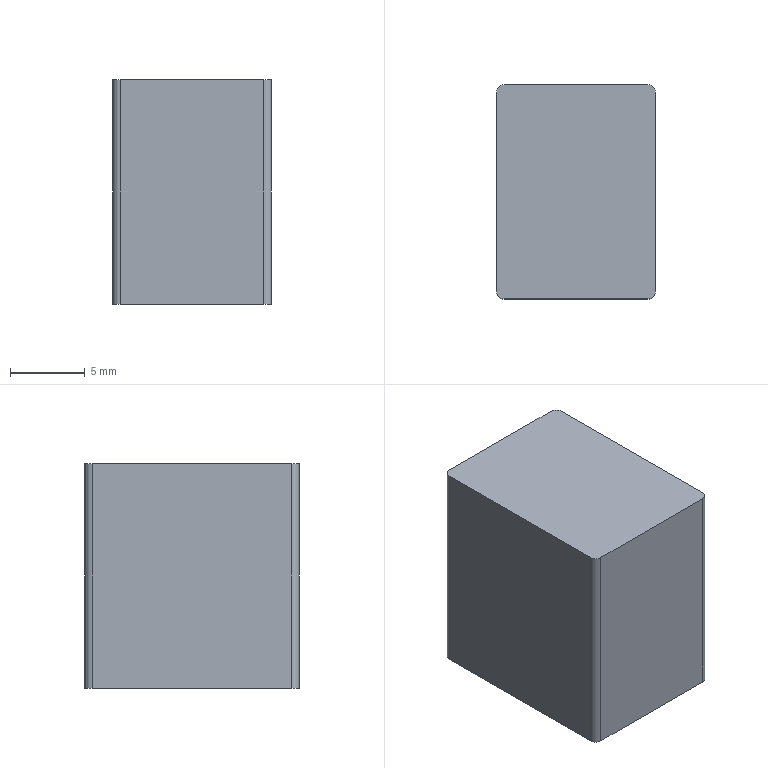Part | NX | features BREP 1 | 1 solid | 10 faces | box 10.615 x 14.326 x 15 mm | volume 2278 mm3 | plane 6 | cylinder 4 | commonest cylinder face diameters 1 x4
STEP:
#1=CARTESIAN_POINT('',(-4.808,7.163,-25.6));
#2=VERTEX_POINT('',#1);
#3=CARTESIAN_POINT('',(-5.308,6.663,-25.6));
#4=VERTEX_POINT('',#3);
#5=CARTESIAN_POINT('',(-4.808,6.663,-25.6));
#6=DIRECTION('',(0.,0.,1.));
#7=DIRECTION('',(1.,0.,0.));
#8=AXIS2_PLACEMENT_3D('',#5,#6,#7);
#9=CIRCLE('',#8,0.5);
#10=EDGE_CURVE('',#2,#4,#9,.T.);
#11=ORIENTED_EDGE('',*,*,#10,.F.);
#12=CARTESIAN_POINT('',(-4.808,7.163,-40.6));
#13=VERTEX_POINT('',#12);
#14=CARTESIAN_POINT('',(-4.808,7.163,-40.6));
#15=DIRECTION('',(0.,0.,1.));
#16=VECTOR('',#15,1000.);
#17=LINE('',#14,#16);
#18=EDGE_CURVE('',#13,#2,#17,.T.);
#19=ORIENTED_EDGE('',*,*,#18,.F.);
#20=CARTESIAN_POINT('',(-5.308,6.663,-40.6));
#21=VERTEX_POINT('',#20);
#22=CARTESIAN_POINT('',(-4.808,6.663,-40.6));
#23=DIRECTION('',(0.,0.,1.));
#24=DIRECTION('',(1.,0.,0.));
#25=AXIS2_PLACEMENT_3D('',#22,#23,#24);
#26=CIRCLE('',#25,0.5);
#27=EDGE_CURVE('',#13,#21,#26,.T.);
#28=ORIENTED_EDGE('',*,*,#27,.T.);
#29=CARTESIAN_POINT('',(-5.308,6.663,-40.6));
#30=DIRECTION('',(0.,0.,1.));
#31=VECTOR('',#30,1000.);
#32=LINE('',#29,#31);
#33=EDGE_CURVE('',#21,#4,#32,.T.);
#34=ORIENTED_EDGE('',*,*,#33,.T.);
#35=EDGE_LOOP('',(#11,#19,#28,#34));
#36=FACE_BOUND('',#35,.T.);
#37=CARTESIAN_POINT('',(-4.808,6.663,-40.6));
#38=DIRECTION('',(0.,0.,1.));
#39=DIRECTION('',(-1.,0.,0.));
#40=AXIS2_PLACEMENT_3D('',#37,#38,#39);
#41=CYLINDRICAL_SURFACE('',#40,0.5);
#42=ADVANCED_FACE('',(#36),#41,.T.);
#43=CARTESIAN_POINT('',(-5.308,-6.663,-25.6));
#44=VERTEX_POINT('',#43);
#45=CARTESIAN_POINT('',(-5.308,-6.663,-25.6));
#46=DIRECTION('',(0.,1.,0.));
#47=VECTOR('',#46,1000.);
#48=LINE('',#45,#47);
#49=EDGE_CURVE('',#44,#4,#48,.T.);
#50=ORIENTED_EDGE('',*,*,#49,.T.);
#51=ORIENTED_EDGE('',*,*,#33,.F.);
#52=CARTESIAN_POINT('',(-5.308,-6.663,-40.6));
#53=VERTEX_POINT('',#52);
#54=CARTESIAN_POINT('',(-5.308,-6.663,-40.6));
#55=DIRECTION('',(0.,1.,0.));
#56=VECTOR('',#55,1000.);
#57=LINE('',#54,#56);
#58=EDGE_CURVE('',#53,#21,#57,.T.);
#59=ORIENTED_EDGE('',*,*,#58,.F.);
#60=CARTESIAN_POINT('',(-5.308,-6.663,-40.6));
#61=DIRECTION('',(0.,0.,1.));
#62=VECTOR('',#61,1000.);
#63=LINE('',#60,#62);
#64=EDGE_CURVE('',#53,#44,#63,.T.);
#65=ORIENTED_EDGE('',*,*,#64,.T.);
#66=EDGE_LOOP('',(#50,#51,#59,#65));
#67=FACE_BOUND('',#66,.T.);
#68=CARTESIAN_POINT('',(-5.308,-6.663,-40.6));
#69=DIRECTION('',(1.,0.,0.));
#70=DIRECTION('',(0.,0.,1.));
#71=AXIS2_PLACEMENT_3D('',#68,#69,#70);
#72=PLANE('',#71);
#73=ADVANCED_FACE('',(#67),#72,.F.);
#74=CARTESIAN_POINT('',(-4.808,-7.163,-25.6));
#75=VERTEX_POINT('',#74);
#76=CARTESIAN_POINT('',(-4.808,-6.663,-25.6));
#77=DIRECTION('',(0.,0.,1.));
#78=DIRECTION('',(1.,0.,0.));
#79=AXIS2_PLACEMENT_3D('',#76,#77,#78);
#80=CIRCLE('',#79,0.5);
#81=EDGE_CURVE('',#44,#75,#80,.T.);
#82=ORIENTED_EDGE('',*,*,#81,.F.);
#83=ORIENTED_EDGE('',*,*,#64,.F.);
#84=CARTESIAN_POINT('',(-4.808,-7.163,-40.6));
#85=VERTEX_POINT('',#84);
#86=CARTESIAN_POINT('',(-4.808,-6.663,-40.6));
#87=DIRECTION('',(0.,0.,1.));
#88=DIRECTION('',(1.,0.,0.));
#89=AXIS2_PLACEMENT_3D('',#86,#87,#88);
#90=CIRCLE('',#89,0.5);
#91=EDGE_CURVE('',#53,#85,#90,.T.);
#92=ORIENTED_EDGE('',*,*,#91,.T.);
#93=CARTESIAN_POINT('',(-4.808,-7.163,-40.6));
#94=DIRECTION('',(0.,0.,1.));
#95=VECTOR('',#94,1000.);
#96=LINE('',#93,#95);
#97=EDGE_CURVE('',#85,#75,#96,.T.);
#98=ORIENTED_EDGE('',*,*,#97,.T.);
#99=EDGE_LOOP('',(#82,#83,#92,#98));
#100=FACE_BOUND('',#99,.T.);
#101=CARTESIAN_POINT('',(-4.808,-6.663,-40.6));
#102=DIRECTION('',(0.,0.,1.));
#103=DIRECTION('',(-1.,0.,0.));
#104=AXIS2_PLACEMENT_3D('',#101,#102,#103);
#105=CYLINDRICAL_SURFACE('',#104,0.5);
#106=ADVANCED_FACE('',(#100),#105,.T.);
#107=CARTESIAN_POINT('',(4.808,-7.163,-25.6));
#108=VERTEX_POINT('',#107);
#109=CARTESIAN_POINT('',(4.808,-7.163,-25.6));
#110=DIRECTION('',(-1.,0.,0.));
#111=VECTOR('',#110,1000.);
#112=LINE('',#109,#111);
#113=EDGE_CURVE('',#108,#75,#112,.T.);
#114=ORIENTED_EDGE('',*,*,#113,.T.);
#115=ORIENTED_EDGE('',*,*,#97,.F.);
#116=CARTESIAN_POINT('',(4.808,-7.163,-40.6));
#117=VERTEX_POINT('',#116);
#118=CARTESIAN_POINT('',(4.808,-7.163,-40.6));
#119=DIRECTION('',(-1.,0.,0.));
#120=VECTOR('',#119,1000.);
#121=LINE('',#118,#120);
#122=EDGE_CURVE('',#117,#85,#121,.T.);
#123=ORIENTED_EDGE('',*,*,#122,.F.);
#124=CARTESIAN_POINT('',(4.808,-7.163,-40.6));
#125=DIRECTION('',(0.,0.,1.));
#126=VECTOR('',#125,1000.);
#127=LINE('',#124,#126);
#128=EDGE_CURVE('',#117,#108,#127,.T.);
#129=ORIENTED_EDGE('',*,*,#128,.T.);
#130=EDGE_LOOP('',(#114,#115,#123,#129));
#131=FACE_BOUND('',#130,.T.);
#132=CARTESIAN_POINT('',(4.808,-7.163,-40.6));
#133=DIRECTION('',(0.,1.,0.));
#134=DIRECTION('',(0.,0.,-1.));
#135=AXIS2_PLACEMENT_3D('',#132,#133,#134);
#136=PLANE('',#135);
#137=ADVANCED_FACE('',(#131),#136,.F.);
#138=CARTESIAN_POINT('',(5.308,-6.663,-25.6));
#139=VERTEX_POINT('',#138);
#140=CARTESIAN_POINT('',(4.808,-6.663,-25.6));
#141=DIRECTION('',(0.,0.,1.));
#142=DIRECTION('',(1.,0.,0.));
#143=AXIS2_PLACEMENT_3D('',#140,#141,#142);
#144=CIRCLE('',#143,0.5);
#145=EDGE_CURVE('',#108,#139,#144,.T.);
#146=ORIENTED_EDGE('',*,*,#145,.F.);
#147=ORIENTED_EDGE('',*,*,#128,.F.);
#148=CARTESIAN_POINT('',(5.308,-6.663,-40.6));
#149=VERTEX_POINT('',#148);
#150=CARTESIAN_POINT('',(4.808,-6.663,-40.6));
#151=DIRECTION('',(0.,0.,1.));
#152=DIRECTION('',(1.,0.,0.));
#153=AXIS2_PLACEMENT_3D('',#150,#151,#152);
#154=CIRCLE('',#153,0.5);
#155=EDGE_CURVE('',#117,#149,#154,.T.);
#156=ORIENTED_EDGE('',*,*,#155,.T.);
#157=CARTESIAN_POINT('',(5.308,-6.663,-40.6));
#158=DIRECTION('',(0.,0.,1.));
#159=VECTOR('',#158,1000.);
#160=LINE('',#157,#159);
#161=EDGE_CURVE('',#149,#139,#160,.T.);
#162=ORIENTED_EDGE('',*,*,#161,.T.);
#163=EDGE_LOOP('',(#146,#147,#156,#162));
#164=FACE_BOUND('',#163,.T.);
#165=CARTESIAN_POINT('',(4.808,-6.663,-40.6));
#166=DIRECTION('',(0.,0.,1.));
#167=DIRECTION('',(-1.,0.,0.));
#168=AXIS2_PLACEMENT_3D('',#165,#166,#167);
#169=CYLINDRICAL_SURFACE('',#168,0.5);
#170=ADVANCED_FACE('',(#164),#169,.T.);
#171=CARTESIAN_POINT('',(5.308,6.663,-25.6));
#172=VERTEX_POINT('',#171);
#173=CARTESIAN_POINT('',(5.308,6.663,-25.6));
#174=DIRECTION('',(0.,-1.,0.));
#175=VECTOR('',#174,1000.);
#176=LINE('',#173,#175);
#177=EDGE_CURVE('',#172,#139,#176,.T.);
#178=ORIENTED_EDGE('',*,*,#177,.T.);
#179=ORIENTED_EDGE('',*,*,#161,.F.);
#180=CARTESIAN_POINT('',(5.308,6.663,-40.6));
#181=VERTEX_POINT('',#180);
#182=CARTESIAN_POINT('',(5.308,6.663,-40.6));
#183=DIRECTION('',(0.,-1.,0.));
#184=VECTOR('',#183,1000.);
#185=LINE('',#182,#184);
#186=EDGE_CURVE('',#181,#149,#185,.T.);
#187=ORIENTED_EDGE('',*,*,#186,.F.);
#188=CARTESIAN_POINT('',(5.308,6.663,-40.6));
#189=DIRECTION('',(0.,0.,1.));
#190=VECTOR('',#189,1000.);
#191=LINE('',#188,#190);
#192=EDGE_CURVE('',#181,#172,#191,.T.);
#193=ORIENTED_EDGE('',*,*,#192,.T.);
#194=EDGE_LOOP('',(#178,#179,#187,#193));
#195=FACE_BOUND('',#194,.T.);
#196=CARTESIAN_POINT('',(5.308,6.663,-40.6));
#197=DIRECTION('',(-1.,0.,0.));
#198=DIRECTION('',(0.,0.,-1.));
#199=AXIS2_PLACEMENT_3D('',#196,#197,#198);
#200=PLANE('',#199);
#201=ADVANCED_FACE('',(#195),#200,.F.);
#202=CARTESIAN_POINT('',(4.808,7.163,-25.6));
#203=VERTEX_POINT('',#202);
#204=CARTESIAN_POINT('',(4.808,6.663,-25.6));
#205=DIRECTION('',(0.,0.,1.));
#206=DIRECTION('',(1.,0.,0.));
#207=AXIS2_PLACEMENT_3D('',#204,#205,#206);
#208=CIRCLE('',#207,0.5);
#209=EDGE_CURVE('',#172,#203,#208,.T.);
#210=ORIENTED_EDGE('',*,*,#209,.F.);
#211=ORIENTED_EDGE('',*,*,#192,.F.);
#212=CARTESIAN_POINT('',(4.808,7.163,-40.6));
#213=VERTEX_POINT('',#212);
#214=CARTESIAN_POINT('',(4.808,6.663,-40.6));
#215=DIRECTION('',(0.,0.,1.));
#216=DIRECTION('',(1.,0.,0.));
#217=AXIS2_PLACEMENT_3D('',#214,#215,#216);
#218=CIRCLE('',#217,0.5);
#219=EDGE_CURVE('',#181,#213,#218,.T.);
#220=ORIENTED_EDGE('',*,*,#219,.T.);
#221=CARTESIAN_POINT('',(4.808,7.163,-40.6));
#222=DIRECTION('',(0.,0.,1.));
#223=VECTOR('',#222,1000.);
#224=LINE('',#221,#223);
#225=EDGE_CURVE('',#213,#203,#224,.T.);
#226=ORIENTED_EDGE('',*,*,#225,.T.);
#227=EDGE_LOOP('',(#210,#211,#220,#226));
#228=FACE_BOUND('',#227,.T.);
#229=CARTESIAN_POINT('',(4.808,6.663,-40.6));
#230=DIRECTION('',(0.,0.,1.));
#231=DIRECTION('',(-1.,0.,0.));
#232=AXIS2_PLACEMENT_3D('',#229,#230,#231);
#233=CYLINDRICAL_SURFACE('',#232,0.5);
#234=ADVANCED_FACE('',(#228),#233,.T.);
#235=CARTESIAN_POINT('',(-4.808,7.163,-25.6));
#236=DIRECTION('',(1.,0.,0.));
#237=VECTOR('',#236,1000.);
#238=LINE('',#235,#237);
#239=EDGE_CURVE('',#2,#203,#238,.T.);
#240=ORIENTED_EDGE('',*,*,#239,.T.);
#241=ORIENTED_EDGE('',*,*,#225,.F.);
#242=CARTESIAN_POINT('',(-4.808,7.163,-40.6));
#243=DIRECTION('',(1.,0.,0.));
#244=VECTOR('',#243,1000.);
#245=LINE('',#242,#244);
#246=EDGE_CURVE('',#13,#213,#245,.T.);
#247=ORIENTED_EDGE('',*,*,#246,.F.);
#248=ORIENTED_EDGE('',*,*,#18,.T.);
#249=EDGE_LOOP('',(#240,#241,#247,#248));
#250=FACE_BOUND('',#249,.T.);
#251=CARTESIAN_POINT('',(-4.808,7.163,-40.6));
#252=DIRECTION('',(0.,-1.,0.));
#253=DIRECTION('',(0.,0.,1.));
#254=AXIS2_PLACEMENT_3D('',#251,#252,#253);
#255=PLANE('',#254);
#256=ADVANCED_FACE('',(#250),#255,.F.);
#257=ORIENTED_EDGE('',*,*,#27,.F.);
#258=ORIENTED_EDGE('',*,*,#246,.T.);
#259=ORIENTED_EDGE('',*,*,#219,.F.);
#260=ORIENTED_EDGE('',*,*,#186,.T.);
#261=ORIENTED_EDGE('',*,*,#155,.F.);
#262=ORIENTED_EDGE('',*,*,#122,.T.);
#263=ORIENTED_EDGE('',*,*,#91,.F.);
#264=ORIENTED_EDGE('',*,*,#58,.T.);
#265=EDGE_LOOP('',(#257,#258,#259,#260,#261,#262,#263,#264));
#266=FACE_BOUND('',#265,.T.);
#267=CARTESIAN_POINT('',(-4.808,6.663,-40.6));
#268=DIRECTION('',(0.,0.,1.));
#269=DIRECTION('',(-1.,0.,0.));
#270=AXIS2_PLACEMENT_3D('',#267,#268,#269);
#271=PLANE('',#270);
#272=ADVANCED_FACE('',(#266),#271,.F.);
#273=ORIENTED_EDGE('',*,*,#10,.T.);
#274=ORIENTED_EDGE('',*,*,#49,.F.);
#275=ORIENTED_EDGE('',*,*,#81,.T.);
#276=ORIENTED_EDGE('',*,*,#113,.F.);
#277=ORIENTED_EDGE('',*,*,#145,.T.);
#278=ORIENTED_EDGE('',*,*,#177,.F.);
#279=ORIENTED_EDGE('',*,*,#209,.T.);
#280=ORIENTED_EDGE('',*,*,#239,.F.);
#281=EDGE_LOOP('',(#273,#274,#275,#276,#277,#278,#279,#280));
#282=FACE_BOUND('',#281,.T.);
#283=CARTESIAN_POINT('',(-4.808,6.663,-25.6));
#284=DIRECTION('',(0.,0.,1.));
#285=DIRECTION('',(-1.,0.,0.));
#286=AXIS2_PLACEMENT_3D('',#283,#284,#285);
#287=PLANE('',#286);
#288=ADVANCED_FACE('',(#282),#287,.T.);
#289=CLOSED_SHELL('',(#42,#73,#106,#137,#170,#201,#234,#256,#272,#288));
#290=MANIFOLD_SOLID_BREP('',#289);
#291=(LENGTH_UNIT()NAMED_UNIT(*)SI_UNIT(.MILLI.,.METRE.));
#292=UNCERTAINTY_MEASURE_WITH_UNIT(LENGTH_MEASURE(0.00001),#291,'','');
#293=(NAMED_UNIT(*)PLANE_ANGLE_UNIT()SI_UNIT($,.RADIAN.));
#294=(NAMED_UNIT(*)SI_UNIT($,.STERADIAN.)SOLID_ANGLE_UNIT());
#295=(GEOMETRIC_REPRESENTATION_CONTEXT(3)GLOBAL_UNCERTAINTY_ASSIGNED_CONTEXT((#292))GLOBAL_UNIT_ASSIGNED_CONTEXT((#291,#293,#294))REPRESENTATION_CONTEXT('',''));
#296=ADVANCED_BREP_SHAPE_REPRESENTATION('',(#290),#295);